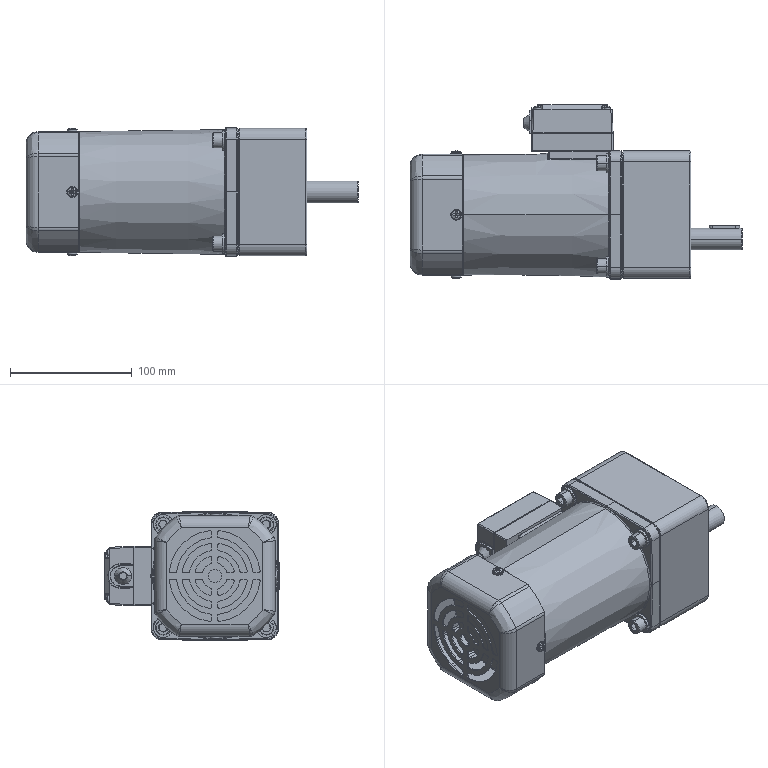Part | SolidWorks | features BaseBody 4 | 4 solids | 1555 faces | box 273 x 143.386 x 105.972 mm | volume 1078601 mm3 | spline 597 | cylinder 462 | plane 429 | cone 59 | torus 8 | commonest cylinder face diameters 0.5 x64 3 x54 4 x44 8 x44 1 x24 2 x17